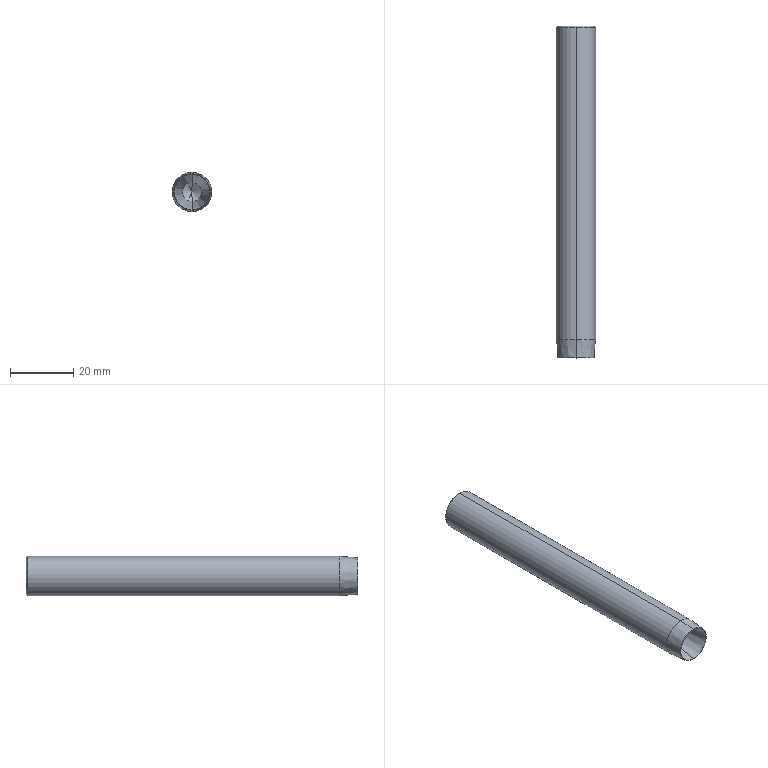Part | STEP file | PN_0058 | 1 solid | 18 faces | box 12.5 x 105 x 12.5 mm | volume 10895 mm3 | cone 10 | cylinder 6 | plane 2 | commonest cylinder face diameters 6 x2 6.8 x2 12.5 x2
STEP:
#1=CARTESIAN_POINT('',(0.,0.,0.));
#2=DIRECTION('',(0.,0.,1.));
#3=DIRECTION('',(1.,0.,0.));
#4=AXIS2_PLACEMENT_3D('',#1,#2,#3);
#5=CARTESIAN_POINT('',(0.,85.25,3.4));
#6=VERTEX_POINT('',#5);
#7=CARTESIAN_POINT('',(0.,105.,3.4));
#8=VERTEX_POINT('',#7);
#9=CARTESIAN_POINT('',(0.,105.,3.4));
#10=DIRECTION('',(0.,1.,0.));
#11=VECTOR('',#10,1.);
#12=LINE('',#9,#11);
#13=CARTESIAN_POINT('',(0.,105.,0.));
#14=DIRECTION('',(0.,1.,0.));
#15=DIRECTION('',(0.,0.,1.));
#16=AXIS2_PLACEMENT_3D('',#13,#14,#15);
#17=CYLINDRICAL_SURFACE('',#16,3.4);
#18=CARTESIAN_POINT('',(6.283,0.));
#19=DIRECTION('',(0.,1.));
#20=VECTOR('',#19,1.);
#21=LINE('',#18,#20);
#22=(GEOMETRIC_REPRESENTATION_CONTEXT(2)PARAMETRIC_REPRESENTATION_CONTEXT()REPRESENTATION_CONTEXT('',''));
#23=DEFINITIONAL_REPRESENTATION('',(#21),#22);
#24=PCURVE('',#17,#23);
#25=CARTESIAN_POINT('',(0.,105.,0.));
#26=DIRECTION('',(0.,1.,0.));
#27=DIRECTION('',(0.,0.,1.));
#28=AXIS2_PLACEMENT_3D('',#25,#26,#27);
#29=CYLINDRICAL_SURFACE('',#28,3.4);
#30=CARTESIAN_POINT('',(0.,0.));
#31=DIRECTION('',(0.,1.));
#32=VECTOR('',#31,1.);
#33=LINE('',#30,#32);
#34=(GEOMETRIC_REPRESENTATION_CONTEXT(2)PARAMETRIC_REPRESENTATION_CONTEXT()REPRESENTATION_CONTEXT('',''));
#35=DEFINITIONAL_REPRESENTATION('',(#33),#34);
#36=PCURVE('',#29,#35);
#37=SURFACE_CURVE('',#12,(#24,#36),.PCURVE_S1.);
#38=EDGE_CURVE('',#6,#8,#37,.T.);
#39=ORIENTED_EDGE('',*,*,#38,.T.);
#40=CARTESIAN_POINT('',(0.,105.,-3.4));
#41=VERTEX_POINT('',#40);
#42=CARTESIAN_POINT('',(0.,105.,0.));
#43=DIRECTION('',(0.,1.,0.));
#44=DIRECTION('',(0.,0.,1.));
#45=AXIS2_PLACEMENT_3D('',#42,#43,#44);
#46=CIRCLE('',#45,3.4);
#47=CARTESIAN_POINT('',(0.,0.));
#48=DIRECTION('',(1.,0.));
#49=VECTOR('',#48,1.);
#50=LINE('',#47,#49);
#51=(GEOMETRIC_REPRESENTATION_CONTEXT(2)PARAMETRIC_REPRESENTATION_CONTEXT()REPRESENTATION_CONTEXT('',''));
#52=DEFINITIONAL_REPRESENTATION('',(#50),#51);
#53=PCURVE('',#17,#52);
#54=CARTESIAN_POINT('',(0.,105.,0.));
#55=DIRECTION('',(0.,1.,0.));
#56=DIRECTION('',(0.,0.,1.));
#57=AXIS2_PLACEMENT_3D('',#54,#55,#56);
#58=PLANE('',#57);
#59=CARTESIAN_POINT('',(0.,0.));
#60=DIRECTION('',(1.,0.));
#61=AXIS2_PLACEMENT_2D('',#59,#60);
#62=CIRCLE('',#61,3.4);
#63=(GEOMETRIC_REPRESENTATION_CONTEXT(2)PARAMETRIC_REPRESENTATION_CONTEXT()REPRESENTATION_CONTEXT('',''));
#64=DEFINITIONAL_REPRESENTATION('',(#62),#63);
#65=PCURVE('',#58,#64);
#66=SURFACE_CURVE('',#46,(#53,#65),.PCURVE_S1.);
#67=EDGE_CURVE('',#41,#8,#66,.T.);
#68=ORIENTED_EDGE('',*,*,#67,.F.);
#69=CARTESIAN_POINT('',(0.,85.25,-3.4));
#70=VERTEX_POINT('',#69);
#71=CARTESIAN_POINT('',(0.,105.,-3.4));
#72=DIRECTION('',(0.,1.,0.));
#73=VECTOR('',#72,1.);
#74=LINE('',#71,#73);
#75=CARTESIAN_POINT('',(3.142,0.));
#76=DIRECTION('',(0.,1.));
#77=VECTOR('',#76,1.);
#78=LINE('',#75,#77);
#79=(GEOMETRIC_REPRESENTATION_CONTEXT(2)PARAMETRIC_REPRESENTATION_CONTEXT()REPRESENTATION_CONTEXT('',''));
#80=DEFINITIONAL_REPRESENTATION('',(#78),#79);
#81=PCURVE('',#17,#80);
#82=CARTESIAN_POINT('',(3.142,0.));
#83=DIRECTION('',(0.,1.));
#84=VECTOR('',#83,1.);
#85=LINE('',#82,#84);
#86=(GEOMETRIC_REPRESENTATION_CONTEXT(2)PARAMETRIC_REPRESENTATION_CONTEXT()REPRESENTATION_CONTEXT('',''));
#87=DEFINITIONAL_REPRESENTATION('',(#85),#86);
#88=PCURVE('',#29,#87);
#89=SURFACE_CURVE('',#74,(#81,#88),.PCURVE_S1.);
#90=EDGE_CURVE('',#70,#41,#89,.T.);
#91=ORIENTED_EDGE('',*,*,#90,.F.);
#92=CARTESIAN_POINT('',(0.,85.25,0.));
#93=DIRECTION('',(0.,1.,0.));
#94=DIRECTION('',(0.,0.,1.));
#95=AXIS2_PLACEMENT_3D('',#92,#93,#94);
#96=CIRCLE('',#95,3.4);
#97=CARTESIAN_POINT('',(0.,-19.75));
#98=DIRECTION('',(1.,0.));
#99=VECTOR('',#98,1.);
#100=LINE('',#97,#99);
#101=(GEOMETRIC_REPRESENTATION_CONTEXT(2)PARAMETRIC_REPRESENTATION_CONTEXT()REPRESENTATION_CONTEXT('',''));
#102=DEFINITIONAL_REPRESENTATION('',(#100),#101);
#103=PCURVE('',#17,#102);
#104=CARTESIAN_POINT('',(0.,85.25,0.));
#105=DIRECTION('',(0.,1.,0.));
#106=DIRECTION('',(0.,0.,1.));
#107=AXIS2_PLACEMENT_3D('',#104,#105,#106);
#108=CONICAL_SURFACE('',#107,3.4,1.03);
#109=CARTESIAN_POINT('',(0.,0.));
#110=DIRECTION('',(1.,0.));
#111=VECTOR('',#110,1.);
#112=LINE('',#109,#111);
#113=(GEOMETRIC_REPRESENTATION_CONTEXT(2)PARAMETRIC_REPRESENTATION_CONTEXT()REPRESENTATION_CONTEXT('',''));
#114=DEFINITIONAL_REPRESENTATION('',(#112),#113);
#115=PCURVE('',#108,#114);
#116=SURFACE_CURVE('',#96,(#103,#115),.PCURVE_S1.);
#117=EDGE_CURVE('',#70,#6,#116,.T.);
#118=ORIENTED_EDGE('',*,*,#117,.T.);
#119=EDGE_LOOP('',(#39,#68,#91,#118));
#120=FACE_BOUND('',#119,.F.);
#121=ADVANCED_FACE('',(#120),#17,.F.);
#122=ORIENTED_EDGE('',*,*,#117,.F.);
#123=CARTESIAN_POINT('',(0.,83.207,0.));
#124=VERTEX_POINT('',#123);
#125=CARTESIAN_POINT('',(0.,85.25,-3.4));
#126=DIRECTION('',(0.,0.515,-0.8572));
#127=VECTOR('',#126,1.);
#128=LINE('',#125,#127);
#129=CARTESIAN_POINT('',(3.142,-2.043));
#130=CARTESIAN_POINT('',(3.142,-2.012));
#131=CARTESIAN_POINT('',(3.142,-1.95));
#132=CARTESIAN_POINT('',(3.142,-1.857));
#133=CARTESIAN_POINT('',(3.142,-1.764));
#134=CARTESIAN_POINT('',(3.142,-1.671));
#135=CARTESIAN_POINT('',(3.142,-1.579));
#136=CARTESIAN_POINT('',(3.142,-1.486));
#137=CARTESIAN_POINT('',(3.142,-1.393));
#138=CARTESIAN_POINT('',(3.142,-1.3));
#139=CARTESIAN_POINT('',(3.142,-1.207));
#140=CARTESIAN_POINT('',(3.142,-1.114));
#141=CARTESIAN_POINT('',(3.142,-1.021));
#142=CARTESIAN_POINT('',(3.142,-0.9286));
#143=CARTESIAN_POINT('',(3.142,-0.8357));
#144=CARTESIAN_POINT('',(3.142,-0.7429));
#145=CARTESIAN_POINT('',(3.142,-0.65));
#146=CARTESIAN_POINT('',(3.142,-0.5572));
#147=CARTESIAN_POINT('',(3.142,-0.4643));
#148=CARTESIAN_POINT('',(3.142,-0.3714));
#149=CARTESIAN_POINT('',(3.142,-0.2786));
#150=CARTESIAN_POINT('',(3.142,-0.1857));
#151=CARTESIAN_POINT('',(3.142,-0.09286));
#152=CARTESIAN_POINT('',(3.142,-0.03095));
#153=CARTESIAN_POINT('',(3.142,0.));
#154=B_SPLINE_CURVE_WITH_KNOTS('',3,(#129,#130,#131,#132,#133,#134,#135,#136,#137,#138,#139,#140,#141,#142,#143,#144,#145,#146,#147,#148,#149,#150,#151,#152,#153),.UNSPECIFIED.,.F.,.F.,(4,1,1,1,1,1,1,1,1,1,1,1,1,1,1,1,1,1,1,1,1,1,4),(-3.967,-3.786,-3.606,-3.426,-3.245,-3.065,-2.885,-2.704,-2.524,-2.344,-2.164,-1.983,-1.803,-1.623,-1.442,-1.262,-1.082,-0.9015,-0.7212,-0.5409,-0.3606,-0.1803,0.),.UNSPECIFIED.);
#155=(GEOMETRIC_REPRESENTATION_CONTEXT(2)PARAMETRIC_REPRESENTATION_CONTEXT()REPRESENTATION_CONTEXT('',''));
#156=DEFINITIONAL_REPRESENTATION('',(#154),#155);
#157=PCURVE('',#108,#156);
#158=CARTESIAN_POINT('',(0.,85.25,0.));
#159=DIRECTION('',(0.,1.,0.));
#160=DIRECTION('',(0.,0.,1.));
#161=AXIS2_PLACEMENT_3D('',#158,#159,#160);
#162=CONICAL_SURFACE('',#161,3.4,1.03);
#163=CARTESIAN_POINT('',(3.142,-2.043));
#164=CARTESIAN_POINT('',(3.142,-2.012));
#165=CARTESIAN_POINT('',(3.142,-1.95));
#166=CARTESIAN_POINT('',(3.142,-1.857));
#167=CARTESIAN_POINT('',(3.142,-1.764));
#168=CARTESIAN_POINT('',(3.142,-1.671));
#169=CARTESIAN_POINT('',(3.142,-1.579));
#170=CARTESIAN_POINT('',(3.142,-1.486));
#171=CARTESIAN_POINT('',(3.142,-1.393));
#172=CARTESIAN_POINT('',(3.142,-1.3));
#173=CARTESIAN_POINT('',(3.142,-1.207));
#174=CARTESIAN_POINT('',(3.142,-1.114));
#175=CARTESIAN_POINT('',(3.142,-1.021));
#176=CARTESIAN_POINT('',(3.142,-0.9286));
#177=CARTESIAN_POINT('',(3.142,-0.8357));
#178=CARTESIAN_POINT('',(3.142,-0.7429));
#179=CARTESIAN_POINT('',(3.142,-0.65));
#180=CARTESIAN_POINT('',(3.142,-0.5572));
#181=CARTESIAN_POINT('',(3.142,-0.4643));
#182=CARTESIAN_POINT('',(3.142,-0.3714));
#183=CARTESIAN_POINT('',(3.142,-0.2786));
#184=CARTESIAN_POINT('',(3.142,-0.1857));
#185=CARTESIAN_POINT('',(3.142,-0.09286));
#186=CARTESIAN_POINT('',(3.142,-0.03095));
#187=CARTESIAN_POINT('',(3.142,0.));
#188=B_SPLINE_CURVE_WITH_KNOTS('',3,(#163,#164,#165,#166,#167,#168,#169,#170,#171,#172,#173,#174,#175,#176,#177,#178,#179,#180,#181,#182,#183,#184,#185,#186,#187),.UNSPECIFIED.,.F.,.F.,(4,1,1,1,1,1,1,1,1,1,1,1,1,1,1,1,1,1,1,1,1,1,4),(-3.967,-3.786,-3.606,-3.426,-3.245,-3.065,-2.885,-2.704,-2.524,-2.344,-2.164,-1.983,-1.803,-1.623,-1.442,-1.262,-1.082,-0.9015,-0.7212,-0.5409,-0.3606,-0.1803,0.),.UNSPECIFIED.);
#189=(GEOMETRIC_REPRESENTATION_CONTEXT(2)PARAMETRIC_REPRESENTATION_CONTEXT()REPRESENTATION_CONTEXT('',''));
#190=DEFINITIONAL_REPRESENTATION('',(#188),#189);
#191=PCURVE('',#162,#190);
#192=SURFACE_CURVE('',#128,(#157,#191),.PCURVE_S1.);
#193=EDGE_CURVE('',#124,#70,#192,.T.);
#194=ORIENTED_EDGE('',*,*,#193,.F.);
#195=CARTESIAN_POINT('',(0.,85.25,3.4));
#196=DIRECTION('',(0.,0.515,0.8572));
#197=VECTOR('',#196,1.);
#198=LINE('',#195,#197);
#199=CARTESIAN_POINT('',(6.283,-2.043));
#200=CARTESIAN_POINT('',(6.283,-2.012));
#201=CARTESIAN_POINT('',(6.283,-1.95));
#202=CARTESIAN_POINT('',(6.283,-1.857));
#203=CARTESIAN_POINT('',(6.283,-1.764));
#204=CARTESIAN_POINT('',(6.283,-1.671));
#205=CARTESIAN_POINT('',(6.283,-1.579));
#206=CARTESIAN_POINT('',(6.283,-1.486));
#207=CARTESIAN_POINT('',(6.283,-1.393));
#208=CARTESIAN_POINT('',(6.283,-1.3));
#209=CARTESIAN_POINT('',(6.283,-1.207));
#210=CARTESIAN_POINT('',(6.283,-1.114));
#211=CARTESIAN_POINT('',(6.283,-1.021));
#212=CARTESIAN_POINT('',(6.283,-0.9286));
#213=CARTESIAN_POINT('',(6.283,-0.8357));
#214=CARTESIAN_POINT('',(6.283,-0.7429));
#215=CARTESIAN_POINT('',(6.283,-0.65));
#216=CARTESIAN_POINT('',(6.283,-0.5572));
#217=CARTESIAN_POINT('',(6.283,-0.4643));
#218=CARTESIAN_POINT('',(6.283,-0.3714));
#219=CARTESIAN_POINT('',(6.283,-0.2786));
#220=CARTESIAN_POINT('',(6.283,-0.1857));
#221=CARTESIAN_POINT('',(6.283,-0.09286));
#222=CARTESIAN_POINT('',(6.283,-0.03095));
#223=CARTESIAN_POINT('',(6.283,0.));
#224=B_SPLINE_CURVE_WITH_KNOTS('',3,(#199,#200,#201,#202,#203,#204,#205,#206,#207,#208,#209,#210,#211,#212,#213,#214,#215,#216,#217,#218,#219,#220,#221,#222,#223),.UNSPECIFIED.,.F.,.F.,(4,1,1,1,1,1,1,1,1,1,1,1,1,1,1,1,1,1,1,1,1,1,4),(-3.967,-3.786,-3.606,-3.426,-3.245,-3.065,-2.885,-2.704,-2.524,-2.344,-2.164,-1.983,-1.803,-1.623,-1.442,-1.262,-1.082,-0.9015,-0.7212,-0.5409,-0.3606,-0.1803,0.),.UNSPECIFIED.);
#225=(GEOMETRIC_REPRESENTATION_CONTEXT(2)PARAMETRIC_REPRESENTATION_CONTEXT()REPRESENTATION_CONTEXT('',''));
#226=DEFINITIONAL_REPRESENTATION('',(#224),#225);
#227=PCURVE('',#108,#226);
#228=CARTESIAN_POINT('',(0.,-2.043));
#229=CARTESIAN_POINT('',(0.,-2.012));
#230=CARTESIAN_POINT('',(0.,-1.95));
#231=CARTESIAN_POINT('',(0.,-1.857));
#232=CARTESIAN_POINT('',(0.,-1.764));
#233=CARTESIAN_POINT('',(0.,-1.671));
#234=CARTESIAN_POINT('',(0.,-1.579));
#235=CARTESIAN_POINT('',(0.,-1.486));
#236=CARTESIAN_POINT('',(0.,-1.393));
#237=CARTESIAN_POINT('',(0.,-1.3));
#238=CARTESIAN_POINT('',(0.,-1.207));
#239=CARTESIAN_POINT('',(0.,-1.114));
#240=CARTESIAN_POINT('',(0.,-1.021));
#241=CARTESIAN_POINT('',(0.,-0.9286));
#242=CARTESIAN_POINT('',(0.,-0.8357));
#243=CARTESIAN_POINT('',(0.,-0.7429));
#244=CARTESIAN_POINT('',(0.,-0.65));
#245=CARTESIAN_POINT('',(0.,-0.5572));
#246=CARTESIAN_POINT('',(0.,-0.4643));
#247=CARTESIAN_POINT('',(0.,-0.3714));
#248=CARTESIAN_POINT('',(0.,-0.2786));
#249=CARTESIAN_POINT('',(0.,-0.1857));
#250=CARTESIAN_POINT('',(0.,-0.09286));
#251=CARTESIAN_POINT('',(0.,-0.03095));
#252=CARTESIAN_POINT('',(0.,0.));
#253=B_SPLINE_CURVE_WITH_KNOTS('',3,(#228,#229,#230,#231,#232,#233,#234,#235,#236,#237,#238,#239,#240,#241,#242,#243,#244,#245,#246,#247,#248,#249,#250,#251,#252),.UNSPECIFIED.,.F.,.F.,(4,1,1,1,1,1,1,1,1,1,1,1,1,1,1,1,1,1,1,1,1,1,4),(-3.967,-3.786,-3.606,-3.426,-3.245,-3.065,-2.885,-2.704,-2.524,-2.344,-2.164,-1.983,-1.803,-1.623,-1.442,-1.262,-1.082,-0.9015,-0.7212,-0.5409,-0.3606,-0.1803,0.),.UNSPECIFIED.);
#254=(GEOMETRIC_REPRESENTATION_CONTEXT(2)PARAMETRIC_REPRESENTATION_CONTEXT()REPRESENTATION_CONTEXT('',''));
#255=DEFINITIONAL_REPRESENTATION('',(#253),#254);
#256=PCURVE('',#162,#255);
#257=SURFACE_CURVE('',#198,(#227,#256),.PCURVE_S1.);
#258=EDGE_CURVE('',#124,#6,#257,.T.);
#259=ORIENTED_EDGE('',*,*,#258,.T.);
#260=EDGE_LOOP('',(#122,#194,#259));
#261=FACE_BOUND('',#260,.F.);
#262=ADVANCED_FACE('',(#261),#108,.F.);
#263=CARTESIAN_POINT('',(0.,105.,5.75));
#264=VERTEX_POINT('',#263);
#265=CARTESIAN_POINT('',(0.,105.,-5.75));
#266=VERTEX_POINT('',#265);
#267=CARTESIAN_POINT('',(0.,105.,0.));
#268=DIRECTION('',(0.,1.,0.));
#269=DIRECTION('',(0.,0.,1.));
#270=AXIS2_PLACEMENT_3D('',#267,#268,#269);
#271=CIRCLE('',#270,5.75);
#272=CARTESIAN_POINT('',(0.,105.,0.));
#273=DIRECTION('',(0.,-1.,0.));
#274=DIRECTION('',(0.,0.,-1.));
#275=AXIS2_PLACEMENT_3D('',#272,#273,#274);
#276=CONICAL_SURFACE('',#275,5.75,0.7854);
#277=CARTESIAN_POINT('',(3.142,0.));
#278=DIRECTION('',(-1.,0.));
#279=VECTOR('',#278,1.);
#280=LINE('',#277,#279);
#281=(GEOMETRIC_REPRESENTATION_CONTEXT(2)PARAMETRIC_REPRESENTATION_CONTEXT()REPRESENTATION_CONTEXT('',''));
#282=DEFINITIONAL_REPRESENTATION('',(#280),#281);
#283=PCURVE('',#276,#282);
#284=CARTESIAN_POINT('',(0.,0.));
#285=DIRECTION('',(1.,0.));
#286=AXIS2_PLACEMENT_2D('',#284,#285);
#287=CIRCLE('',#286,5.75);
#288=(GEOMETRIC_REPRESENTATION_CONTEXT(2)PARAMETRIC_REPRESENTATION_CONTEXT()REPRESENTATION_CONTEXT('',''));
#289=DEFINITIONAL_REPRESENTATION('',(#287),#288);
#290=PCURVE('',#58,#289);
#291=SURFACE_CURVE('',#271,(#283,#290),.PCURVE_S1.);
#292=EDGE_CURVE('',#264,#266,#291,.T.);
#293=ORIENTED_EDGE('',*,*,#292,.F.);
#294=CARTESIAN_POINT('',(0.,104.5,6.25));
#295=VERTEX_POINT('',#294);
#296=CARTESIAN_POINT('',(0.,105.,5.75));
#297=DIRECTION('',(0.,-0.7071,0.7071));
#298=VECTOR('',#297,1.);
#299=LINE('',#296,#298);
#300=CARTESIAN_POINT('',(3.142,0.));
#301=DIRECTION('',(0.,1.));
#302=VECTOR('',#301,1.);
#303=LINE('',#300,#302);
#304=(GEOMETRIC_REPRESENTATION_CONTEXT(2)PARAMETRIC_REPRESENTATION_CONTEXT()REPRESENTATION_CONTEXT('',''));
#305=DEFINITIONAL_REPRESENTATION('',(#303),#304);
#306=PCURVE('',#276,#305);
#307=CARTESIAN_POINT('',(0.,105.,0.));
#308=DIRECTION('',(0.,-1.,0.));
#309=DIRECTION('',(0.,0.,-1.));
#310=AXIS2_PLACEMENT_3D('',#307,#308,#309);
#311=CONICAL_SURFACE('',#310,5.75,0.7854);
#312=CARTESIAN_POINT('',(3.142,0.));
#313=DIRECTION('',(0.,1.));
#314=VECTOR('',#313,1.);
#315=LINE('',#312,#314);
#316=(GEOMETRIC_REPRESENTATION_CONTEXT(2)PARAMETRIC_REPRESENTATION_CONTEXT()REPRESENTATION_CONTEXT('',''));
#317=DEFINITIONAL_REPRESENTATION('',(#315),#316);
#318=PCURVE('',#311,#317);
#319=SURFACE_CURVE('',#299,(#306,#318),.PCURVE_S1.);
#320=EDGE_CURVE('',#264,#295,#319,.T.);
#321=ORIENTED_EDGE('',*,*,#320,.T.);
#322=CARTESIAN_POINT('',(0.,104.5,-6.25));
#323=VERTEX_POINT('',#322);
#324=CARTESIAN_POINT('',(0.,104.5,0.));
#325=DIRECTION('',(0.,-1.,0.));
#326=DIRECTION('',(0.,0.,1.));
#327=AXIS2_PLACEMENT_3D('',#324,#325,#326);
#328=CIRCLE('',#327,6.25);
#329=CARTESIAN_POINT('',(-3.142,0.5));
#330=DIRECTION('',(1.,0.));
#331=VECTOR('',#330,1.);
#332=LINE('',#329,#331);
#333=(GEOMETRIC_REPRESENTATION_CONTEXT(2)PARAMETRIC_REPRESENTATION_CONTEXT()REPRESENTATION_CONTEXT('',''));
#334=DEFINITIONAL_REPRESENTATION('',(#332),#333);
#335=PCURVE('',#276,#334);
#336=CARTESIAN_POINT('',(0.,105.,0.));
#337=DIRECTION('',(0.,-1.,0.));
#338=DIRECTION('',(0.,0.,-1.));
#339=AXIS2_PLACEMENT_3D('',#336,#337,#338);
#340=CYLINDRICAL_SURFACE('',#339,6.25);
#341=CARTESIAN_POINT('',(-3.142,0.5));
#342=DIRECTION('',(1.,0.));
#343=VECTOR('',#342,1.);
#344=LINE('',#341,#343);
#345=(GEOMETRIC_REPRESENTATION_CONTEXT(2)PARAMETRIC_REPRESENTATION_CONTEXT()REPRESENTATION_CONTEXT('',''));
#346=DEFINITIONAL_REPRESENTATION('',(#344),#345);
#347=PCURVE('',#340,#346);
#348=SURFACE_CURVE('',#328,(#335,#347),.PCURVE_S1.);
#349=EDGE_CURVE('',#323,#295,#348,.T.);
#350=ORIENTED_EDGE('',*,*,#349,.F.);
#351=CARTESIAN_POINT('',(0.,105.,-5.75));
#352=DIRECTION('',(0.,-0.7071,-0.7071));
#353=VECTOR('',#352,1.);
#354=LINE('',#351,#353);
#355=CARTESIAN_POINT('',(0.,0.));
#356=DIRECTION('',(0.,1.));
#357=VECTOR('',#356,1.);
#358=LINE('',#355,#357);
#359=(GEOMETRIC_REPRESENTATION_CONTEXT(2)PARAMETRIC_REPRESENTATION_CONTEXT()REPRESENTATION_CONTEXT('',''));
#360=DEFINITIONAL_REPRESENTATION('',(#358),#359);
#361=PCURVE('',#276,#360);
#362=CARTESIAN_POINT('',(6.283,0.));
#363=DIRECTION('',(0.,1.));
#364=VECTOR('',#363,1.);
#365=LINE('',#362,#364);
#366=(GEOMETRIC_REPRESENTATION_CONTEXT(2)PARAMETRIC_REPRESENTATION_CONTEXT()REPRESENTATION_CONTEXT('',''));
#367=DEFINITIONAL_REPRESENTATION('',(#365),#366);
#368=PCURVE('',#311,#367);
#369=SURFACE_CURVE('',#354,(#361,#368),.PCURVE_S1.);
#370=EDGE_CURVE('',#266,#323,#369,.T.);
#371=ORIENTED_EDGE('',*,*,#370,.F.);
#372=EDGE_LOOP('',(#293,#321,#350,#371));
#373=FACE_BOUND('',#372,.T.);
#374=ADVANCED_FACE('',(#373),#276,.T.);
#375=CARTESIAN_POINT('',(0.,14.745,-3.));
#376=VERTEX_POINT('',#375);
#377=CARTESIAN_POINT('',(0.,0.,-5.6));
#378=VERTEX_POINT('',#377);
#379=CARTESIAN_POINT('',(0.,14.745,-3.));
#380=DIRECTION('',(0.,-0.9848,-0.1736));
#381=VECTOR('',#380,1.);
#382=LINE('',#379,#381);
#383=CARTESIAN_POINT('',(0.,14.745,0.));
#384=DIRECTION('',(0.,-1.,0.));
#385=DIRECTION('',(0.,0.,-1.));
#386=AXIS2_PLACEMENT_3D('',#383,#384,#385);
#387=CONICAL_SURFACE('',#386,3.,0.1745);
#388=CARTESIAN_POINT('',(6.283,0.));
#389=DIRECTION('',(0.,1.));
#390=VECTOR('',#389,1.);
#391=LINE('',#388,#390);
#392=(GEOMETRIC_REPRESENTATION_CONTEXT(2)PARAMETRIC_REPRESENTATION_CONTEXT()REPRESENTATION_CONTEXT('',''));
#393=DEFINITIONAL_REPRESENTATION('',(#391),#392);
#394=PCURVE('',#387,#393);
#395=CARTESIAN_POINT('',(0.,14.745,0.));
#396=DIRECTION('',(0.,-1.,0.));
#397=DIRECTION('',(0.,0.,-1.));
#398=AXIS2_PLACEMENT_3D('',#395,#396,#397);
#399=CONICAL_SURFACE('',#398,3.,0.1745);
#400=CARTESIAN_POINT('',(0.,0.));
#401=DIRECTION('',(0.,1.));
#402=VECTOR('',#401,1.);
#403=LINE('',#400,#402);
#404=(GEOMETRIC_REPRESENTATION_CONTEXT(2)PARAMETRIC_REPRESENTATION_CONTEXT()REPRESENTATION_CONTEXT('',''));
#405=DEFINITIONAL_REPRESENTATION('',(#403),#404);
#406=PCURVE('',#399,#405);
#407=SURFACE_CURVE('',#382,(#394,#406),.PCURVE_S1.);
#408=EDGE_CURVE('',#376,#378,#407,.T.);
#409=ORIENTED_EDGE('',*,*,#408,.T.);
#410=CARTESIAN_POINT('',(0.,0.,5.6));
#411=VERTEX_POINT('',#410);
#412=CARTESIAN_POINT('',(0.,0.,0.));
#413=DIRECTION('',(0.,1.,0.));
#414=DIRECTION('',(0.,0.,1.));
#415=AXIS2_PLACEMENT_3D('',#412,#413,#414);
#416=CIRCLE('',#415,5.6);
#417=CARTESIAN_POINT('',(9.425,14.745));
#418=DIRECTION('',(-1.,0.));
#419=VECTOR('',#418,1.);
#420=LINE('',#417,#419);
#421=(GEOMETRIC_REPRESENTATION_CONTEXT(2)PARAMETRIC_REPRESENTATION_CONTEXT()REPRESENTATION_CONTEXT('',''));
#422=DEFINITIONAL_REPRESENTATION('',(#420),#421);
#423=PCURVE('',#387,#422);
#424=CARTESIAN_POINT('',(0.,0.,0.));
#425=DIRECTION('',(0.,1.,0.));
#426=DIRECTION('',(0.,0.,1.));
#427=AXIS2_PLACEMENT_3D('',#424,#425,#426);
#428=PLANE('',#427);
#429=CARTESIAN_POINT('',(0.,0.));
#430=DIRECTION('',(1.,0.));
#431=AXIS2_PLACEMENT_2D('',#429,#430);
#432=CIRCLE('',#431,5.6);
#433=(GEOMETRIC_REPRESENTATION_CONTEXT(2)PARAMETRIC_REPRESENTATION_CONTEXT()REPRESENTATION_CONTEXT('',''));
#434=DEFINITIONAL_REPRESENTATION('',(#432),#433);
#435=PCURVE('',#428,#434);
#436=SURFACE_CURVE('',#416,(#423,#435),.PCURVE_S1.);
#437=EDGE_CURVE('',#378,#411,#436,.T.);
#438=ORIENTED_EDGE('',*,*,#437,.T.);
#439=CARTESIAN_POINT('',(0.,14.745,3.));
#440=VERTEX_POINT('',#439);
#441=CARTESIAN_POINT('',(0.,14.745,3.));
#442=DIRECTION('',(0.,-0.9848,0.1736));
#443=VECTOR('',#442,1.);
#444=LINE('',#441,#443);
#445=CARTESIAN_POINT('',(3.142,0.));
#446=DIRECTION('',(0.,1.));
#447=VECTOR('',#446,1.);
#448=LINE('',#445,#447);
#449=(GEOMETRIC_REPRESENTATION_CONTEXT(2)PARAMETRIC_REPRESENTATION_CONTEXT()REPRESENTATION_CONTEXT('',''));
#450=DEFINITIONAL_REPRESENTATION('',(#448),#449);
#451=PCURVE('',#387,#450);
#452=CARTESIAN_POINT('',(3.142,0.));
#453=DIRECTION('',(0.,1.));
#454=VECTOR('',#453,1.);
#455=LINE('',#452,#454);
#456=(GEOMETRIC_REPRESENTATION_CONTEXT(2)PARAMETRIC_REPRESENTATION_CONTEXT()REPRESENTATION_CONTEXT('',''));
#457=DEFINITIONAL_REPRESENTATION('',(#455),#456);
#458=PCURVE('',#399,#457);
#459=SURFACE_CURVE('',#444,(#451,#458),.PCURVE_S1.);
#460=EDGE_CURVE('',#440,#411,#459,.T.);
#461=ORIENTED_EDGE('',*,*,#460,.F.);
#462=CARTESIAN_POINT('',(0.,14.745,0.));
#463=DIRECTION('',(0.,-1.,0.));
#464=DIRECTION('',(0.,0.,1.));
#465=AXIS2_PLACEMENT_3D('',#462,#463,#464);
#466=CIRCLE('',#465,3.);
#467=CARTESIAN_POINT('',(3.142,0.));
#468=DIRECTION('',(1.,0.));
#469=VECTOR('',#468,1.);
#470=LINE('',#467,#469);
#471=(GEOMETRIC_REPRESENTATION_CONTEXT(2)PARAMETRIC_REPRESENTATION_CONTEXT()REPRESENTATION_CONTEXT('',''));
#472=DEFINITIONAL_REPRESENTATION('',(#470),#471);
#473=PCURVE('',#387,#472);
#474=CARTESIAN_POINT('',(0.,0.,0.));
#475=DIRECTION('',(0.,-1.,0.));
#476=DIRECTION('',(0.,0.,-1.));
#477=AXIS2_PLACEMENT_3D('',#474,#475,#476);
#478=CYLINDRICAL_SURFACE('',#477,3.);
#479=CARTESIAN_POINT('',(3.142,-14.745));
#480=DIRECTION('',(1.,0.));
#481=VECTOR('',#480,1.);
#482=LINE('',#479,#481);
#483=(GEOMETRIC_REPRESENTATION_CONTEXT(2)PARAMETRIC_REPRESENTATION_CONTEXT()REPRESENTATION_CONTEXT('',''));
#484=DEFINITIONAL_REPRESENTATION('',(#482),#483);
#485=PCURVE('',#478,#484);
#486=SURFACE_CURVE('',#466,(#473,#485),.PCURVE_S1.);
#487=EDGE_CURVE('',#440,#376,#486,.T.);
#488=ORIENTED_EDGE('',*,*,#487,.T.);
#489=EDGE_LOOP('',(#409,#438,#461,#488));
#490=FACE_BOUND('',#489,.F.);
#491=ADVANCED_FACE('',(#490),#387,.F.);
#492=CARTESIAN_POINT('',(0.,0.,-5.75));
#493=VERTEX_POINT('',#492);
#494=CARTESIAN_POINT('',(0.,0.,5.75));
#495=VERTEX_POINT('',#494);
#496=CARTESIAN_POINT('',(0.,0.,0.));
#497=DIRECTION('',(0.,-1.,0.));
#498=DIRECTION('',(0.,0.,1.));
#499=AXIS2_PLACEMENT_3D('',#496,#497,#498);
#500=CIRCLE('',#499,5.75);
#501=CARTESIAN_POINT('',(0.,5.715,0.));
#502=DIRECTION('',(0.,1.,0.));
#503=DIRECTION('',(0.,0.,1.));
#504=AXIS2_PLACEMENT_3D('',#501,#502,#503);
#505=CONICAL_SURFACE('',#504,6.25,0.08727);
#506=CARTESIAN_POINT('',(6.283,-5.715));
#507=DIRECTION('',(-1.,0.));
#508=VECTOR('',#507,1.);
#509=LINE('',#506,#508);
#510=(GEOMETRIC_REPRESENTATION_CONTEXT(2)PARAMETRIC_REPRESENTATION_CONTEXT()REPRESENTATION_CONTEXT('',''));
#511=DEFINITIONAL_REPRESENTATION('',(#509),#510);
#512=PCURVE('',#505,#511);
#513=CARTESIAN_POINT('',(5.75,0.));
#514=CARTESIAN_POINT('',(5.75,-9.959));
#515=CARTESIAN_POINT('',(-2.875,-4.98));
#516=CARTESIAN_POINT('',(-11.5,0.));
#517=CARTESIAN_POINT('',(-2.875,4.98));
#518=CARTESIAN_POINT('',(5.75,9.959));
#519=CARTESIAN_POINT('',(5.75,0.));
#520=(BOUNDED_CURVE()B_SPLINE_CURVE(2,(#513,#514,#515,#516,#517,#518,#519),.UNSPECIFIED.,.T.,.F.)B_SPLINE_CURVE_WITH_KNOTS((1,2,2,2,2,1),(-2.094,0.,2.094,4.189,6.283,8.378),.UNSPECIFIED.)CURVE()GEOMETRIC_REPRESENTATION_ITEM()RATIONAL_B_SPLINE_CURVE((1.,0.5,1.,0.5,1.,0.5,1.))REPRESENTATION_ITEM(''));
#521=(GEOMETRIC_REPRESENTATION_CONTEXT(2)PARAMETRIC_REPRESENTATION_CONTEXT()REPRESENTATION_CONTEXT('',''));
#522=DEFINITIONAL_REPRESENTATION('',(#520),#521);
#523=PCURVE('',#428,#522);
#524=SURFACE_CURVE('',#500,(#512,#523),.PCURVE_S1.);
#525=EDGE_CURVE('',#493,#495,#524,.T.);
#526=ORIENTED_EDGE('',*,*,#525,.F.);
#527=CARTESIAN_POINT('',(0.,5.715,-6.25));
#528=VERTEX_POINT('',#527);
#529=CARTESIAN_POINT('',(0.,5.715,-6.25));
#530=DIRECTION('',(0.,0.9962,-0.08716));
#531=VECTOR('',#530,1.);
#532=LINE('',#529,#531);
#533=CARTESIAN_POINT('',(3.142,0.));
#534=DIRECTION('',(0.,1.));
#535=VECTOR('',#534,1.);
#536=LINE('',#533,#535);
#537=(GEOMETRIC_REPRESENTATION_CONTEXT(2)PARAMETRIC_REPRESENTATION_CONTEXT()REPRESENTATION_CONTEXT('',''));
#538=DEFINITIONAL_REPRESENTATION('',(#536),#537);
#539=PCURVE('',#505,#538);
#540=CARTESIAN_POINT('',(0.,5.715,0.));
#541=DIRECTION('',(0.,1.,0.));
#542=DIRECTION('',(0.,0.,1.));
#543=AXIS2_PLACEMENT_3D('',#540,#541,#542);
#544=CONICAL_SURFACE('',#543,6.25,0.08727);
#545=CARTESIAN_POINT('',(3.142,0.));
#546=DIRECTION('',(0.,1.));
#547=VECTOR('',#546,1.);
#548=LINE('',#545,#547);
#549=(GEOMETRIC_REPRESENTATION_CONTEXT(2)PARAMETRIC_REPRESENTATION_CONTEXT()REPRESENTATION_CONTEXT('',''));
#550=DEFINITIONAL_REPRESENTATION('',(#548),#549);
#551=PCURVE('',#544,#550);
#552=SURFACE_CURVE('',#532,(#539,#551),.PCURVE_S1.);
#553=EDGE_CURVE('',#493,#528,#552,.T.);
#554=ORIENTED_EDGE('',*,*,#553,.T.);
#555=CARTESIAN_POINT('',(0.,5.715,6.25));
#556=VERTEX_POINT('',#555);
#557=CARTESIAN_POINT('',(0.,5.715,0.));
#558=DIRECTION('',(0.,1.,0.));
#559=DIRECTION('',(0.,0.,1.));
#560=AXIS2_PLACEMENT_3D('',#557,#558,#559);
#561=CIRCLE('',#560,6.25);
#562=CARTESIAN_POINT('',(0.,0.));
#563=DIRECTION('',(1.,0.));
#564=VECTOR('',#563,1.);
#565=LINE('',#562,#564);
#566=(GEOMETRIC_REPRESENTATION_CONTEXT(2)PARAMETRIC_REPRESENTATION_CONTEXT()REPRESENTATION_CONTEXT('',''));
#567=DEFINITIONAL_REPRESENTATION('',(#565),#566);
#568=PCURVE('',#505,#567);
#569=CARTESIAN_POINT('',(3.142,99.285));
#570=DIRECTION('',(-1.,0.));
#571=VECTOR('',#570,1.);
#572=LINE('',#569,#571);
#573=(GEOMETRIC_REPRESENTATION_CONTEXT(2)PARAMETRIC_REPRESENTATION_CONTEXT()REPRESENTATION_CONTEXT('',''));
#574=DEFINITIONAL_REPRESENTATION('',(#572),#573);
#575=PCURVE('',#340,#574);
#576=SURFACE_CURVE('',#561,(#568,#575),.PCURVE_S1.);
#577=EDGE_CURVE('',#556,#528,#576,.T.);
#578=ORIENTED_EDGE('',*,*,#577,.F.);
#579=CARTESIAN_POINT('',(0.,5.715,6.25));
#580=DIRECTION('',(0.,0.9962,0.08716));
#581=VECTOR('',#580,1.);
#582=LINE('',#579,#581);
#583=CARTESIAN_POINT('',(0.,0.));
#584=DIRECTION('',(0.,1.));
#585=VECTOR('',#584,1.);
#586=LINE('',#583,#585);
#587=(GEOMETRIC_REPRESENTATION_CONTEXT(2)PARAMETRIC_REPRESENTATION_CONTEXT()REPRESENTATION_CONTEXT('',''));
#588=DEFINITIONAL_REPRESENTATION('',(#586),#587);
#589=PCURVE('',#505,#588);
#590=CARTESIAN_POINT('',(6.283,0.));
#591=DIRECTION('',(0.,1.));
#592=VECTOR('',#591,1.);
#593=LINE('',#590,#592);
#594=(GEOMETRIC_REPRESENTATION_CONTEXT(2)PARAMETRIC_REPRESENTATION_CONTEXT()REPRESENTATION_CONTEXT('',''));
#595=DEFINITIONAL_REPRESENTATION('',(#593),#594);
#596=PCURVE('',#544,#595);
#597=SURFACE_CURVE('',#582,(#589,#596),.PCURVE_S1.);
#598=EDGE_CURVE('',#495,#556,#597,.T.);
#599=ORIENTED_EDGE('',*,*,#598,.F.);
#600=EDGE_LOOP('',(#526,#554,#578,#599));
#601=FACE_BOUND('',#600,.T.);
#602=ADVANCED_FACE('',(#601),#505,.T.);
#603=CARTESIAN_POINT('',(0.,25.,-3.));
#604=VERTEX_POINT('',#603);
#605=CARTESIAN_POINT('',(0.,0.,-3.));
#606=DIRECTION('',(0.,-1.,0.));
#607=VECTOR('',#606,1.);
#608=LINE('',#605,#607);
#609=CARTESIAN_POINT('',(6.283,0.));
#610=DIRECTION('',(0.,1.));
#611=VECTOR('',#610,1.);
#612=LINE('',#609,#611);
#613=(GEOMETRIC_REPRESENTATION_CONTEXT(2)PARAMETRIC_REPRESENTATION_CONTEXT()REPRESENTATION_CONTEXT('',''));
#614=DEFINITIONAL_REPRESENTATION('',(#612),#613);
#615=PCURVE('',#478,#614);
#616=CARTESIAN_POINT('',(0.,0.,0.));
#617=DIRECTION('',(0.,-1.,0.));
#618=DIRECTION('',(0.,0.,-1.));
#619=AXIS2_PLACEMENT_3D('',#616,#617,#618);
#620=CYLINDRICAL_SURFACE('',#619,3.);
#621=CARTESIAN_POINT('',(0.,0.));
#622=DIRECTION('',(0.,1.));
#623=VECTOR('',#622,1.);
#624=LINE('',#621,#623);
#625=(GEOMETRIC_REPRESENTATION_CONTEXT(2)PARAMETRIC_REPRESENTATION_CONTEXT()REPRESENTATION_CONTEXT('',''));
#626=DEFINITIONAL_REPRESENTATION('',(#624),#625);
#627=PCURVE('',#620,#626);
#628=SURFACE_CURVE('',#608,(#615,#627),.PCURVE_S1.);
#629=EDGE_CURVE('',#604,#376,#628,.T.);
#630=ORIENTED_EDGE('',*,*,#629,.T.);
#631=ORIENTED_EDGE('',*,*,#487,.F.);
#632=CARTESIAN_POINT('',(0.,25.,3.));
#633=VERTEX_POINT('',#632);
#634=CARTESIAN_POINT('',(0.,0.,3.));
#635=DIRECTION('',(0.,-1.,0.));
#636=VECTOR('',#635,1.);
#637=LINE('',#634,#636);
#638=CARTESIAN_POINT('',(3.142,0.));
#639=DIRECTION('',(0.,1.));
#640=VECTOR('',#639,1.);
#641=LINE('',#638,#640);
#642=(GEOMETRIC_REPRESENTATION_CONTEXT(2)PARAMETRIC_REPRESENTATION_CONTEXT()REPRESENTATION_CONTEXT('',''));
#643=DEFINITIONAL_REPRESENTATION('',(#641),#642);
#644=PCURVE('',#478,#643);
#645=CARTESIAN_POINT('',(3.142,0.));
#646=DIRECTION('',(0.,1.));
#647=VECTOR('',#646,1.);
#648=LINE('',#645,#647);
#649=(GEOMETRIC_REPRESENTATION_CONTEXT(2)PARAMETRIC_REPRESENTATION_CONTEXT()REPRESENTATION_CONTEXT('',''));
#650=DEFINITIONAL_REPRESENTATION('',(#648),#649);
#651=PCURVE('',#620,#650);
#652=SURFACE_CURVE('',#637,(#644,#651),.PCURVE_S1.);
#653=EDGE_CURVE('',#633,#440,#652,.T.);
#654=ORIENTED_EDGE('',*,*,#653,.F.);
#655=CARTESIAN_POINT('',(0.,25.,0.));
#656=DIRECTION('',(0.,-1.,0.));
#657=DIRECTION('',(0.,0.,-1.));
#658=AXIS2_PLACEMENT_3D('',#655,#656,#657);
#659=CIRCLE('',#658,3.);
#660=CARTESIAN_POINT('',(0.,-25.));
#661=DIRECTION('',(1.,0.));
#662=VECTOR('',#661,1.);
#663=LINE('',#660,#662);
#664=(GEOMETRIC_REPRESENTATION_CONTEXT(2)PARAMETRIC_REPRESENTATION_CONTEXT()REPRESENTATION_CONTEXT('',''));
#665=DEFINITIONAL_REPRESENTATION('',(#663),#664);
#666=PCURVE('',#478,#665);
#667=CARTESIAN_POINT('',(0.,25.,0.));
#668=DIRECTION('',(0.,-1.,0.));
#669=DIRECTION('',(0.,0.,-1.));
#670=AXIS2_PLACEMENT_3D('',#667,#668,#669);
#671=CONICAL_SURFACE('',#670,3.,1.03);
#672=CARTESIAN_POINT('',(0.,0.));
#673=DIRECTION('',(1.,0.));
#674=VECTOR('',#673,1.);
#675=LINE('',#672,#674);
#676=(GEOMETRIC_REPRESENTATION_CONTEXT(2)PARAMETRIC_REPRESENTATION_CONTEXT()REPRESENTATION_CONTEXT('',''));
#677=DEFINITIONAL_REPRESENTATION('',(#675),#676);
#678=PCURVE('',#671,#677);
#679=SURFACE_CURVE('',#659,(#666,#678),.PCURVE_S1.);
#680=EDGE_CURVE('',#633,#604,#679,.T.);
#681=ORIENTED_EDGE('',*,*,#680,.T.);
#682=EDGE_LOOP('',(#630,#631,#654,#681));
#683=FACE_BOUND('',#682,.F.);
#684=ADVANCED_FACE('',(#683),#478,.F.);
#685=ORIENTED_EDGE('',*,*,#680,.F.);
#686=CARTESIAN_POINT('',(0.,26.803,0.));
#687=VERTEX_POINT('',#686);
#688=CARTESIAN_POINT('',(0.,25.,3.));
#689=DIRECTION('',(0.,-0.515,0.8572));
#690=VECTOR('',#689,1.);
#691=LINE('',#688,#690);
#692=CARTESIAN_POINT('',(3.142,0.));
#693=DIRECTION('',(0.,1.));
#694=VECTOR('',#693,1.);
#695=LINE('',#692,#694);
#696=(GEOMETRIC_REPRESENTATION_CONTEXT(2)PARAMETRIC_REPRESENTATION_CONTEXT()REPRESENTATION_CONTEXT('',''));
#697=DEFINITIONAL_REPRESENTATION('',(#695),#696);
#698=PCURVE('',#671,#697);
#699=CARTESIAN_POINT('',(0.,25.,0.));
#700=DIRECTION('',(0.,-1.,0.));
#701=DIRECTION('',(0.,0.,-1.));
#702=AXIS2_PLACEMENT_3D('',#699,#700,#701);
#703=CONICAL_SURFACE('',#702,3.,1.03);
#704=CARTESIAN_POINT('',(3.142,0.));
#705=DIRECTION('',(0.,1.));
#706=VECTOR('',#705,1.);
#707=LINE('',#704,#706);
#708=(GEOMETRIC_REPRESENTATION_CONTEXT(2)PARAMETRIC_REPRESENTATION_CONTEXT()REPRESENTATION_CONTEXT('',''));
#709=DEFINITIONAL_REPRESENTATION('',(#707),#708);
#710=PCURVE('',#703,#709);
#711=SURFACE_CURVE('',#691,(#698,#710),.PCURVE_S1.);
#712=EDGE_CURVE('',#687,#633,#711,.T.);
#713=ORIENTED_EDGE('',*,*,#712,.F.);
#714=CARTESIAN_POINT('',(0.,25.,-3.));
#715=DIRECTION('',(0.,-0.515,-0.8572));
#716=VECTOR('',#715,1.);
#717=LINE('',#714,#716);
#718=CARTESIAN_POINT('',(6.283,0.));
#719=DIRECTION('',(0.,1.));
#720=VECTOR('',#719,1.);
#721=LINE('',#718,#720);
#722=(GEOMETRIC_REPRESENTATION_CONTEXT(2)PARAMETRIC_REPRESENTATION_CONTEXT()REPRESENTATION_CONTEXT('',''));
#723=DEFINITIONAL_REPRESENTATION('',(#721),#722);
#724=PCURVE('',#671,#723);
#725=CARTESIAN_POINT('',(0.,0.));
#726=DIRECTION('',(0.,1.));
#727=VECTOR('',#726,1.);
#728=LINE('',#725,#727);
#729=(GEOMETRIC_REPRESENTATION_CONTEXT(2)PARAMETRIC_REPRESENTATION_CONTEXT()REPRESENTATION_CONTEXT('',''));
#730=DEFINITIONAL_REPRESENTATION('',(#728),#729);
#731=PCURVE('',#703,#730);
#732=SURFACE_CURVE('',#717,(#724,#731),.PCURVE_S1.);
#733=EDGE_CURVE('',#687,#604,#732,.T.);
#734=ORIENTED_EDGE('',*,*,#733,.T.);
#735=EDGE_LOOP('',(#685,#713,#734));
#736=FACE_BOUND('',#735,.F.);
#737=ADVANCED_FACE('',(#736),#671,.F.);
#738=ORIENTED_EDGE('',*,*,#349,.T.);
#739=CARTESIAN_POINT('',(0.,105.,6.25));
#740=DIRECTION('',(0.,-1.,0.));
#741=VECTOR('',#740,1.);
#742=LINE('',#739,#741);
#743=CARTESIAN_POINT('',(3.142,0.));
#744=DIRECTION('',(0.,1.));
#745=VECTOR('',#744,1.);
#746=LINE('',#743,#745);
#747=(GEOMETRIC_REPRESENTATION_CONTEXT(2)PARAMETRIC_REPRESENTATION_CONTEXT()REPRESENTATION_CONTEXT('',''));
#748=DEFINITIONAL_REPRESENTATION('',(#746),#747);
#749=PCURVE('',#340,#748);
#750=CARTESIAN_POINT('',(0.,105.,0.));
#751=DIRECTION('',(0.,-1.,0.));
#752=DIRECTION('',(0.,0.,-1.));
#753=AXIS2_PLACEMENT_3D('',#750,#751,#752);
#754=CYLINDRICAL_SURFACE('',#753,6.25);
#755=CARTESIAN_POINT('',(3.142,0.));
#756=DIRECTION('',(0.,1.));
#757=VECTOR('',#756,1.);
#758=LINE('',#755,#757);
#759=(GEOMETRIC_REPRESENTATION_CONTEXT(2)PARAMETRIC_REPRESENTATION_CONTEXT()REPRESENTATION_CONTEXT('',''));
#760=DEFINITIONAL_REPRESENTATION('',(#758),#759);
#761=PCURVE('',#754,#760);
#762=SURFACE_CURVE('',#742,(#749,#761),.PCURVE_S1.);
#763=EDGE_CURVE('',#295,#556,#762,.T.);
#764=ORIENTED_EDGE('',*,*,#763,.T.);
#765=ORIENTED_EDGE('',*,*,#577,.T.);
#766=CARTESIAN_POINT('',(0.,105.,-6.25));
#767=DIRECTION('',(0.,-1.,0.));
#768=VECTOR('',#767,1.);
#769=LINE('',#766,#768);
#770=CARTESIAN_POINT('',(0.,0.));
#771=DIRECTION('',(0.,1.));
#772=VECTOR('',#771,1.);
#773=LINE('',#770,#772);
#774=(GEOMETRIC_REPRESENTATION_CONTEXT(2)PARAMETRIC_REPRESENTATION_CONTEXT()REPRESENTATION_CONTEXT('',''));
#775=DEFINITIONAL_REPRESENTATION('',(#773),#774);
#776=PCURVE('',#340,#775);
#777=CARTESIAN_POINT('',(6.283,0.));
#778=DIRECTION('',(0.,1.));
#779=VECTOR('',#778,1.);
#780=LINE('',#777,#779);
#781=(GEOMETRIC_REPRESENTATION_CONTEXT(2)PARAMETRIC_REPRESENTATION_CONTEXT()REPRESENTATION_CONTEXT('',''));
#782=DEFINITIONAL_REPRESENTATION('',(#780),#781);
#783=PCURVE('',#754,#782);
#784=SURFACE_CURVE('',#769,(#776,#783),.PCURVE_S1.);
#785=EDGE_CURVE('',#323,#528,#784,.T.);
#786=ORIENTED_EDGE('',*,*,#785,.F.);
#787=EDGE_LOOP('',(#738,#764,#765,#786));
#788=FACE_BOUND('',#787,.T.);
#789=ADVANCED_FACE('',(#788),#340,.T.);
#790=ORIENTED_EDGE('',*,*,#763,.F.);
#791=CARTESIAN_POINT('',(0.,104.5,0.));
#792=DIRECTION('',(0.,-1.,0.));
#793=DIRECTION('',(0.,0.,1.));
#794=AXIS2_PLACEMENT_3D('',#791,#792,#793);
#795=CIRCLE('',#794,6.25);
#796=CARTESIAN_POINT('',(3.142,0.5));
#797=DIRECTION('',(1.,0.));
#798=VECTOR('',#797,1.);
#799=LINE('',#796,#798);
#800=(GEOMETRIC_REPRESENTATION_CONTEXT(2)PARAMETRIC_REPRESENTATION_CONTEXT()REPRESENTATION_CONTEXT('',''));
#801=DEFINITIONAL_REPRESENTATION('',(#799),#800);
#802=PCURVE('',#754,#801);
#803=CARTESIAN_POINT('',(3.142,0.5));
#804=DIRECTION('',(1.,0.));
#805=VECTOR('',#804,1.);
#806=LINE('',#803,#805);
#807=(GEOMETRIC_REPRESENTATION_CONTEXT(2)PARAMETRIC_REPRESENTATION_CONTEXT()REPRESENTATION_CONTEXT('',''));
#808=DEFINITIONAL_REPRESENTATION('',(#806),#807);
#809=PCURVE('',#311,#808);
#810=SURFACE_CURVE('',#795,(#802,#809),.PCURVE_S1.);
#811=EDGE_CURVE('',#295,#323,#810,.T.);
#812=ORIENTED_EDGE('',*,*,#811,.T.);
#813=ORIENTED_EDGE('',*,*,#785,.T.);
#814=CARTESIAN_POINT('',(0.,5.715,0.));
#815=DIRECTION('',(0.,1.,0.));
#816=DIRECTION('',(0.,0.,1.));
#817=AXIS2_PLACEMENT_3D('',#814,#815,#816);
#818=CIRCLE('',#817,6.25);
#819=CARTESIAN_POINT('',(9.425,99.285));
#820=DIRECTION('',(-1.,0.));
#821=VECTOR('',#820,1.);
#822=LINE('',#819,#821);
#823=(GEOMETRIC_REPRESENTATION_CONTEXT(2)PARAMETRIC_REPRESENTATION_CONTEXT()REPRESENTATION_CONTEXT('',''));
#824=DEFINITIONAL_REPRESENTATION('',(#822),#823);
#825=PCURVE('',#754,#824);
#826=CARTESIAN_POINT('',(0.,0.));
#827=DIRECTION('',(1.,0.));
#828=VECTOR('',#827,1.);
#829=LINE('',#826,#828);
#830=(GEOMETRIC_REPRESENTATION_CONTEXT(2)PARAMETRIC_REPRESENTATION_CONTEXT()REPRESENTATION_CONTEXT('',''));
#831=DEFINITIONAL_REPRESENTATION('',(#829),#830);
#832=PCURVE('',#544,#831);
#833=SURFACE_CURVE('',#818,(#825,#832),.PCURVE_S1.);
#834=EDGE_CURVE('',#528,#556,#833,.T.);
#835=ORIENTED_EDGE('',*,*,#834,.T.);
#836=EDGE_LOOP('',(#790,#812,#813,#835));
#837=FACE_BOUND('',#836,.T.);
#838=ADVANCED_FACE('',(#837),#754,.T.);
#839=CARTESIAN_POINT('',(0.,105.,0.));
#840=DIRECTION('',(0.,1.,0.));
#841=DIRECTION('',(0.,0.,1.));
#842=AXIS2_PLACEMENT_3D('',#839,#840,#841);
#843=CIRCLE('',#842,3.4);
#844=CARTESIAN_POINT('',(0.,0.));
#845=DIRECTION('',(1.,0.));
#846=AXIS2_PLACEMENT_2D('',#844,#845);
#847=CIRCLE('',#846,3.4);
#848=(GEOMETRIC_REPRESENTATION_CONTEXT(2)PARAMETRIC_REPRESENTATION_CONTEXT()REPRESENTATION_CONTEXT('',''));
#849=DEFINITIONAL_REPRESENTATION('',(#847),#848);
#850=PCURVE('',#58,#849);
#851=CARTESIAN_POINT('',(0.,0.));
#852=DIRECTION('',(1.,0.));
#853=VECTOR('',#852,1.);
#854=LINE('',#851,#853);
#855=(GEOMETRIC_REPRESENTATION_CONTEXT(2)PARAMETRIC_REPRESENTATION_CONTEXT()REPRESENTATION_CONTEXT('',''));
#856=DEFINITIONAL_REPRESENTATION('',(#854),#855);
#857=PCURVE('',#29,#856);
#858=SURFACE_CURVE('',#843,(#850,#857),.PCURVE_S1.);
#859=EDGE_CURVE('',#8,#41,#858,.T.);
#860=ORIENTED_EDGE('',*,*,#859,.F.);
#861=ORIENTED_EDGE('',*,*,#67,.F.);
#862=EDGE_LOOP('',(#860,#861));
#863=FACE_BOUND('',#862,.T.);
#864=CARTESIAN_POINT('',(0.,105.,0.));
#865=DIRECTION('',(0.,1.,0.));
#866=DIRECTION('',(0.,0.,1.));
#867=AXIS2_PLACEMENT_3D('',#864,#865,#866);
#868=CIRCLE('',#867,5.75);
#869=CARTESIAN_POINT('',(0.,0.));
#870=DIRECTION('',(1.,0.));
#871=AXIS2_PLACEMENT_2D('',#869,#870);
#872=CIRCLE('',#871,5.75);
#873=(GEOMETRIC_REPRESENTATION_CONTEXT(2)PARAMETRIC_REPRESENTATION_CONTEXT()REPRESENTATION_CONTEXT('',''));
#874=DEFINITIONAL_REPRESENTATION('',(#872),#873);
#875=PCURVE('',#58,#874);
#876=CARTESIAN_POINT('',(9.425,0.));
#877=DIRECTION('',(-1.,0.));
#878=VECTOR('',#877,1.);
#879=LINE('',#876,#878);
#880=(GEOMETRIC_REPRESENTATION_CONTEXT(2)PARAMETRIC_REPRESENTATION_CONTEXT()REPRESENTATION_CONTEXT('',''));
#881=DEFINITIONAL_REPRESENTATION('',(#879),#880);
#882=PCURVE('',#311,#881);
#883=SURFACE_CURVE('',#868,(#875,#882),.PCURVE_S1.);
#884=EDGE_CURVE('',#266,#264,#883,.T.);
#885=ORIENTED_EDGE('',*,*,#884,.T.);
#886=ORIENTED_EDGE('',*,*,#292,.T.);
#887=EDGE_LOOP('',(#885,#886));
#888=FACE_BOUND('',#887,.T.);
#889=ADVANCED_FACE('',(#863,#888),#58,.T.);
#890=ORIENTED_EDGE('',*,*,#437,.T.);
#891=CARTESIAN_POINT('',(0.,0.,0.));
#892=DIRECTION('',(0.,1.,0.));
#893=DIRECTION('',(0.,0.,1.));
#894=AXIS2_PLACEMENT_3D('',#891,#892,#893);
#895=CIRCLE('',#894,5.6);
#896=CARTESIAN_POINT('',(0.,0.));
#897=DIRECTION('',(1.,0.));
#898=AXIS2_PLACEMENT_2D('',#896,#897);
#899=CIRCLE('',#898,5.6);
#900=(GEOMETRIC_REPRESENTATION_CONTEXT(2)PARAMETRIC_REPRESENTATION_CONTEXT()REPRESENTATION_CONTEXT('',''));
#901=DEFINITIONAL_REPRESENTATION('',(#899),#900);
#902=PCURVE('',#428,#901);
#903=CARTESIAN_POINT('',(3.142,14.745));
#904=DIRECTION('',(-1.,0.));
#905=VECTOR('',#904,1.);
#906=LINE('',#903,#905);
#907=(GEOMETRIC_REPRESENTATION_CONTEXT(2)PARAMETRIC_REPRESENTATION_CONTEXT()REPRESENTATION_CONTEXT('',''));
#908=DEFINITIONAL_REPRESENTATION('',(#906),#907);
#909=PCURVE('',#399,#908);
#910=SURFACE_CURVE('',#895,(#902,#909),.PCURVE_S1.);
#911=EDGE_CURVE('',#411,#378,#910,.T.);
#912=ORIENTED_EDGE('',*,*,#911,.T.);
#913=EDGE_LOOP('',(#890,#912));
#914=FACE_BOUND('',#913,.T.);
#915=CARTESIAN_POINT('',(0.,0.,0.));
#916=DIRECTION('',(0.,-1.,0.));
#917=DIRECTION('',(0.,0.,1.));
#918=AXIS2_PLACEMENT_3D('',#915,#916,#917);
#919=CIRCLE('',#918,5.75);
#920=CARTESIAN_POINT('',(5.75,0.));
#921=CARTESIAN_POINT('',(5.75,-9.959));
#922=CARTESIAN_POINT('',(-2.875,-4.98));
#923=CARTESIAN_POINT('',(-11.5,0.));
#924=CARTESIAN_POINT('',(-2.875,4.98));
#925=CARTESIAN_POINT('',(5.75,9.959));
#926=CARTESIAN_POINT('',(5.75,0.));
#927=(BOUNDED_CURVE()B_SPLINE_CURVE(2,(#920,#921,#922,#923,#924,#925,#926),.UNSPECIFIED.,.T.,.F.)B_SPLINE_CURVE_WITH_KNOTS((1,2,2,2,2,1),(-2.094,0.,2.094,4.189,6.283,8.378),.UNSPECIFIED.)CURVE()GEOMETRIC_REPRESENTATION_ITEM()RATIONAL_B_SPLINE_CURVE((1.,0.5,1.,0.5,1.,0.5,1.))REPRESENTATION_ITEM(''));
#928=(GEOMETRIC_REPRESENTATION_CONTEXT(2)PARAMETRIC_REPRESENTATION_CONTEXT()REPRESENTATION_CONTEXT('',''));
#929=DEFINITIONAL_REPRESENTATION('',(#927),#928);
#930=PCURVE('',#428,#929);
#931=CARTESIAN_POINT('',(6.283,-5.715));
#932=DIRECTION('',(-1.,0.));
#933=VECTOR('',#932,1.);
#934=LINE('',#931,#933);
#935=(GEOMETRIC_REPRESENTATION_CONTEXT(2)PARAMETRIC_REPRESENTATION_CONTEXT()REPRESENTATION_CONTEXT('',''));
#936=DEFINITIONAL_REPRESENTATION('',(#934),#935);
#937=PCURVE('',#544,#936);
#938=SURFACE_CURVE('',#919,(#930,#937),.PCURVE_S1.);
#939=EDGE_CURVE('',#495,#493,#938,.T.);
#940=ORIENTED_EDGE('',*,*,#939,.T.);
#941=ORIENTED_EDGE('',*,*,#525,.T.);
#942=EDGE_LOOP('',(#940,#941));
#943=FACE_BOUND('',#942,.T.);
#944=ADVANCED_FACE('',(#914,#943),#428,.F.);
#945=CARTESIAN_POINT('',(0.,25.,0.));
#946=DIRECTION('',(0.,-1.,0.));
#947=DIRECTION('',(0.,0.,-1.));
#948=AXIS2_PLACEMENT_3D('',#945,#946,#947);
#949=CIRCLE('',#948,3.);
#950=CARTESIAN_POINT('',(0.,0.));
#951=DIRECTION('',(1.,0.));
#952=VECTOR('',#951,1.);
#953=LINE('',#950,#952);
#954=(GEOMETRIC_REPRESENTATION_CONTEXT(2)PARAMETRIC_REPRESENTATION_CONTEXT()REPRESENTATION_CONTEXT('',''));
#955=DEFINITIONAL_REPRESENTATION('',(#953),#954);
#956=PCURVE('',#703,#955);
#957=CARTESIAN_POINT('',(0.,-25.));
#958=DIRECTION('',(1.,0.));
#959=VECTOR('',#958,1.);
#960=LINE('',#957,#959);
#961=(GEOMETRIC_REPRESENTATION_CONTEXT(2)PARAMETRIC_REPRESENTATION_CONTEXT()REPRESENTATION_CONTEXT('',''));
#962=DEFINITIONAL_REPRESENTATION('',(#960),#961);
#963=PCURVE('',#620,#962);
#964=SURFACE_CURVE('',#949,(#956,#963),.PCURVE_S1.);
#965=EDGE_CURVE('',#604,#633,#964,.T.);
#966=ORIENTED_EDGE('',*,*,#965,.F.);
#967=ORIENTED_EDGE('',*,*,#733,.F.);
#968=ORIENTED_EDGE('',*,*,#712,.T.);
#969=EDGE_LOOP('',(#966,#967,#968));
#970=FACE_BOUND('',#969,.F.);
#971=ADVANCED_FACE('',(#970),#703,.F.);
#972=CARTESIAN_POINT('',(0.,14.745,0.));
#973=DIRECTION('',(0.,-1.,0.));
#974=DIRECTION('',(0.,0.,1.));
#975=AXIS2_PLACEMENT_3D('',#972,#973,#974);
#976=CIRCLE('',#975,3.);
#977=CARTESIAN_POINT('',(-3.142,-14.745));
#978=DIRECTION('',(1.,0.));
#979=VECTOR('',#978,1.);
#980=LINE('',#977,#979);
#981=(GEOMETRIC_REPRESENTATION_CONTEXT(2)PARAMETRIC_REPRESENTATION_CONTEXT()REPRESENTATION_CONTEXT('',''));
#982=DEFINITIONAL_REPRESENTATION('',(#980),#981);
#983=PCURVE('',#620,#982);
#984=CARTESIAN_POINT('',(-3.142,0.));
#985=DIRECTION('',(1.,0.));
#986=VECTOR('',#985,1.);
#987=LINE('',#984,#986);
#988=(GEOMETRIC_REPRESENTATION_CONTEXT(2)PARAMETRIC_REPRESENTATION_CONTEXT()REPRESENTATION_CONTEXT('',''));
#989=DEFINITIONAL_REPRESENTATION('',(#987),#988);
#990=PCURVE('',#399,#989);
#991=SURFACE_CURVE('',#976,(#983,#990),.PCURVE_S1.);
#992=EDGE_CURVE('',#376,#440,#991,.T.);
#993=ORIENTED_EDGE('',*,*,#992,.F.);
#994=ORIENTED_EDGE('',*,*,#629,.F.);
#995=ORIENTED_EDGE('',*,*,#965,.T.);
#996=ORIENTED_EDGE('',*,*,#653,.T.);
#997=EDGE_LOOP('',(#993,#994,#995,#996));
#998=FACE_BOUND('',#997,.F.);
#999=ADVANCED_FACE('',(#998),#620,.F.);
#1000=ORIENTED_EDGE('',*,*,#553,.F.);
#1001=ORIENTED_EDGE('',*,*,#939,.F.);
#1002=ORIENTED_EDGE('',*,*,#598,.T.);
#1003=ORIENTED_EDGE('',*,*,#834,.F.);
#1004=EDGE_LOOP('',(#1000,#1001,#1002,#1003));
#1005=FACE_BOUND('',#1004,.T.);
#1006=ADVANCED_FACE('',(#1005),#544,.T.);
#1007=ORIENTED_EDGE('',*,*,#911,.T.);
#1008=ORIENTED_EDGE('',*,*,#408,.F.);
#1009=ORIENTED_EDGE('',*,*,#992,.T.);
#1010=ORIENTED_EDGE('',*,*,#460,.T.);
#1011=EDGE_LOOP('',(#1007,#1008,#1009,#1010));
#1012=FACE_BOUND('',#1011,.F.);
#1013=ADVANCED_FACE('',(#1012),#399,.F.);
#1014=ORIENTED_EDGE('',*,*,#320,.F.);
#1015=ORIENTED_EDGE('',*,*,#884,.F.);
#1016=ORIENTED_EDGE('',*,*,#370,.T.);
#1017=ORIENTED_EDGE('',*,*,#811,.F.);
#1018=EDGE_LOOP('',(#1014,#1015,#1016,#1017));
#1019=FACE_BOUND('',#1018,.T.);
#1020=ADVANCED_FACE('',(#1019),#311,.T.);
#1021=CARTESIAN_POINT('',(0.,85.25,0.));
#1022=DIRECTION('',(0.,1.,0.));
#1023=DIRECTION('',(0.,0.,1.));
#1024=AXIS2_PLACEMENT_3D('',#1021,#1022,#1023);
#1025=CIRCLE('',#1024,3.4);
#1026=CARTESIAN_POINT('',(0.,0.));
#1027=DIRECTION('',(1.,0.));
#1028=VECTOR('',#1027,1.);
#1029=LINE('',#1026,#1028);
#1030=(GEOMETRIC_REPRESENTATION_CONTEXT(2)PARAMETRIC_REPRESENTATION_CONTEXT()REPRESENTATION_CONTEXT('',''));
#1031=DEFINITIONAL_REPRESENTATION('',(#1029),#1030);
#1032=PCURVE('',#162,#1031);
#1033=CARTESIAN_POINT('',(0.,-19.75));
#1034=DIRECTION('',(1.,0.));
#1035=VECTOR('',#1034,1.);
#1036=LINE('',#1033,#1035);
#1037=(GEOMETRIC_REPRESENTATION_CONTEXT(2)PARAMETRIC_REPRESENTATION_CONTEXT()REPRESENTATION_CONTEXT('',''));
#1038=DEFINITIONAL_REPRESENTATION('',(#1036),#1037);
#1039=PCURVE('',#29,#1038);
#1040=SURFACE_CURVE('',#1025,(#1032,#1039),.PCURVE_S1.);
#1041=EDGE_CURVE('',#6,#70,#1040,.T.);
#1042=ORIENTED_EDGE('',*,*,#1041,.F.);
#1043=ORIENTED_EDGE('',*,*,#258,.F.);
#1044=ORIENTED_EDGE('',*,*,#193,.T.);
#1045=EDGE_LOOP('',(#1042,#1043,#1044));
#1046=FACE_BOUND('',#1045,.F.);
#1047=ADVANCED_FACE('',(#1046),#162,.F.);
#1048=ORIENTED_EDGE('',*,*,#859,.F.);
#1049=ORIENTED_EDGE('',*,*,#38,.F.);
#1050=ORIENTED_EDGE('',*,*,#1041,.T.);
#1051=ORIENTED_EDGE('',*,*,#90,.T.);
#1052=EDGE_LOOP('',(#1048,#1049,#1050,#1051));
#1053=FACE_BOUND('',#1052,.F.);
#1054=ADVANCED_FACE('',(#1053),#29,.F.);
#1055=CLOSED_SHELL('',(#121,#262,#374,#491,#602,#684,#737,#789,#838,#889,#944,#971,#999,#1006,#1013,#1020,#1047,#1054));
#1056=MANIFOLD_SOLID_BREP('',#1055);
#1057=(LENGTH_UNIT()NAMED_UNIT(*)SI_UNIT(.MILLI.,.METRE.));
#1058=UNCERTAINTY_MEASURE_WITH_UNIT(LENGTH_MEASURE(0.0000001),#1057,'','');
#1059=(NAMED_UNIT(*)PLANE_ANGLE_UNIT()SI_UNIT($,.RADIAN.));
#1060=(NAMED_UNIT(*)SI_UNIT($,.STERADIAN.)SOLID_ANGLE_UNIT());
#1061=(GEOMETRIC_REPRESENTATION_CONTEXT(3)GLOBAL_UNCERTAINTY_ASSIGNED_CONTEXT((#1058))GLOBAL_UNIT_ASSIGNED_CONTEXT((#1057,#1059,#1060))REPRESENTATION_CONTEXT('',''));
#1062=ADVANCED_BREP_SHAPE_REPRESENTATION('',(#4,#1056),#1061);